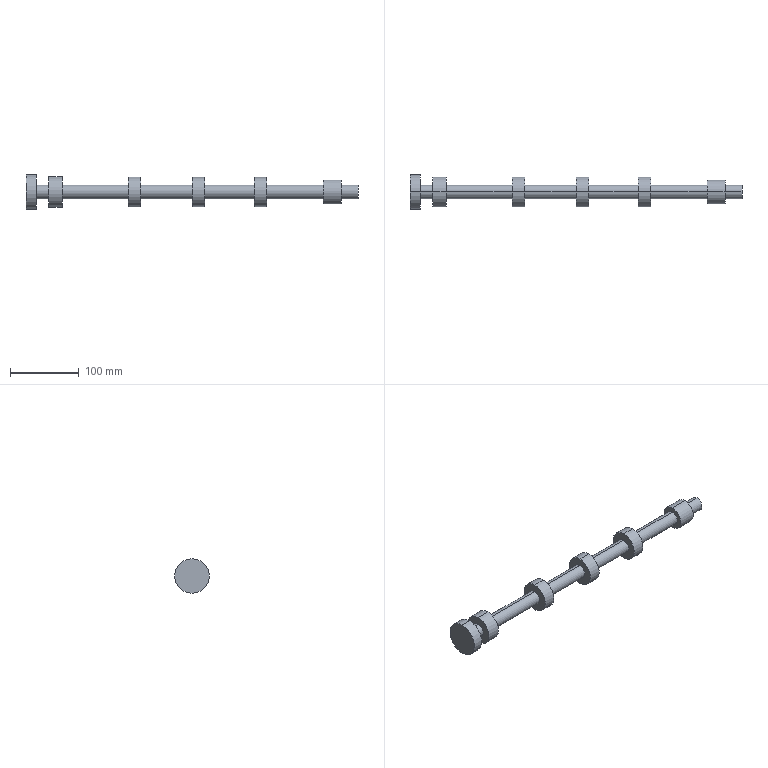Part | SolidWorks | features Revolution 1 | 1 solid | 37 faces | box 482.1 x 50 x 50 mm | volume 277870 mm3 | cylinder 24 | plane 13 | commonest cylinder face diameters 20 x12 34.5 x2 42.8 x2 43.1 x2 43.4 x2 43.7 x2
STEP:
#1=CARTESIAN_POINT('',(-2484.57,0.,10.));
#2=VERTEX_POINT('',#1);
#3=CARTESIAN_POINT('',(-2484.57,0.,-10.));
#4=VERTEX_POINT('',#3);
#5=CARTESIAN_POINT('',(-2484.57,0.,0.));
#6=DIRECTION('',(-1.,0.,0.));
#7=DIRECTION('',(0.,0.,1.));
#8=AXIS2_PLACEMENT_3D('',#5,#6,#7);
#9=CIRCLE('',#8,10.);
#10=EDGE_CURVE('',#2,#4,#9,.T.);
#11=ORIENTED_EDGE('',*,*,#10,.T.);
#12=CARTESIAN_POINT('',(-2509.17,0.,-10.));
#13=VERTEX_POINT('',#12);
#14=CARTESIAN_POINT('',(-2966.67,0.,-10.));
#15=DIRECTION('',(-1.,0.,0.));
#16=VECTOR('',#15,1000.);
#17=LINE('',#14,#16);
#18=EDGE_CURVE('',#4,#13,#17,.T.);
#19=ORIENTED_EDGE('',*,*,#18,.T.);
#20=CARTESIAN_POINT('',(-2509.17,0.,10.));
#21=VERTEX_POINT('',#20);
#22=CARTESIAN_POINT('',(-2509.17,0.,0.));
#23=DIRECTION('',(-1.,0.,0.));
#24=DIRECTION('',(0.,0.,1.));
#25=AXIS2_PLACEMENT_3D('',#22,#23,#24);
#26=CIRCLE('',#25,10.);
#27=EDGE_CURVE('',#21,#13,#26,.T.);
#28=ORIENTED_EDGE('',*,*,#27,.F.);
#29=CARTESIAN_POINT('',(-2966.67,0.,10.));
#30=DIRECTION('',(-1.,0.,0.));
#31=VECTOR('',#30,1000.);
#32=LINE('',#29,#31);
#33=EDGE_CURVE('',#2,#21,#32,.T.);
#34=ORIENTED_EDGE('',*,*,#33,.F.);
#35=EDGE_LOOP('',(#11,#19,#28,#34));
#36=FACE_OUTER_BOUND('',#35,.T.);
#37=CARTESIAN_POINT('',(-2966.67,0.,0.));
#38=DIRECTION('',(-1.,0.,0.));
#39=DIRECTION('',(0.,0.,1.));
#40=AXIS2_PLACEMENT_3D('',#37,#38,#39);
#41=CYLINDRICAL_SURFACE('',#40,10.);
#42=ADVANCED_FACE('',(#36),#41,.T.);
#43=CARTESIAN_POINT('',(-2509.17,0.,17.25));
#44=VERTEX_POINT('',#43);
#45=CARTESIAN_POINT('',(-2509.17,0.,-17.25));
#46=VERTEX_POINT('',#45);
#47=CARTESIAN_POINT('',(-2509.17,0.,0.));
#48=DIRECTION('',(-1.,0.,0.));
#49=DIRECTION('',(0.,0.,1.));
#50=AXIS2_PLACEMENT_3D('',#47,#48,#49);
#51=CIRCLE('',#50,17.25);
#52=EDGE_CURVE('',#44,#46,#51,.T.);
#53=ORIENTED_EDGE('',*,*,#52,.T.);
#54=CARTESIAN_POINT('',(-2535.17,0.,-17.25));
#55=VERTEX_POINT('',#54);
#56=CARTESIAN_POINT('',(-2966.67,0.,-17.25));
#57=DIRECTION('',(-1.,0.,0.));
#58=VECTOR('',#57,1000.);
#59=LINE('',#56,#58);
#60=EDGE_CURVE('',#46,#55,#59,.T.);
#61=ORIENTED_EDGE('',*,*,#60,.T.);
#62=CARTESIAN_POINT('',(-2535.17,0.,17.25));
#63=VERTEX_POINT('',#62);
#64=CARTESIAN_POINT('',(-2535.17,0.,0.));
#65=DIRECTION('',(-1.,0.,0.));
#66=DIRECTION('',(0.,0.,1.));
#67=AXIS2_PLACEMENT_3D('',#64,#65,#66);
#68=CIRCLE('',#67,17.25);
#69=EDGE_CURVE('',#63,#55,#68,.T.);
#70=ORIENTED_EDGE('',*,*,#69,.F.);
#71=CARTESIAN_POINT('',(-2966.67,0.,17.25));
#72=DIRECTION('',(-1.,0.,0.));
#73=VECTOR('',#72,1000.);
#74=LINE('',#71,#73);
#75=EDGE_CURVE('',#44,#63,#74,.T.);
#76=ORIENTED_EDGE('',*,*,#75,.F.);
#77=EDGE_LOOP('',(#53,#61,#70,#76));
#78=FACE_OUTER_BOUND('',#77,.T.);
#79=CARTESIAN_POINT('',(-2966.67,0.,0.));
#80=DIRECTION('',(-1.,0.,0.));
#81=DIRECTION('',(0.,0.,1.));
#82=AXIS2_PLACEMENT_3D('',#79,#80,#81);
#83=CYLINDRICAL_SURFACE('',#82,17.25);
#84=ADVANCED_FACE('',(#78),#83,.T.);
#85=CARTESIAN_POINT('',(-2535.17,0.,10.));
#86=VERTEX_POINT('',#85);
#87=CARTESIAN_POINT('',(-2535.17,0.,-10.));
#88=VERTEX_POINT('',#87);
#89=CARTESIAN_POINT('',(-2535.17,0.,0.));
#90=DIRECTION('',(-1.,0.,0.));
#91=DIRECTION('',(0.,0.,1.));
#92=AXIS2_PLACEMENT_3D('',#89,#90,#91);
#93=CIRCLE('',#92,10.);
#94=EDGE_CURVE('',#86,#88,#93,.T.);
#95=ORIENTED_EDGE('',*,*,#94,.T.);
#96=CARTESIAN_POINT('',(-2617.17,0.,-10.));
#97=VERTEX_POINT('',#96);
#98=CARTESIAN_POINT('',(-2966.67,0.,-10.));
#99=DIRECTION('',(-1.,0.,0.));
#100=VECTOR('',#99,1000.);
#101=LINE('',#98,#100);
#102=EDGE_CURVE('',#88,#97,#101,.T.);
#103=ORIENTED_EDGE('',*,*,#102,.T.);
#104=CARTESIAN_POINT('',(-2617.17,0.,10.));
#105=VERTEX_POINT('',#104);
#106=CARTESIAN_POINT('',(-2617.17,0.,0.));
#107=DIRECTION('',(-1.,0.,0.));
#108=DIRECTION('',(0.,0.,1.));
#109=AXIS2_PLACEMENT_3D('',#106,#107,#108);
#110=CIRCLE('',#109,10.);
#111=EDGE_CURVE('',#105,#97,#110,.T.);
#112=ORIENTED_EDGE('',*,*,#111,.F.);
#113=CARTESIAN_POINT('',(-2966.67,0.,10.));
#114=DIRECTION('',(-1.,0.,0.));
#115=VECTOR('',#114,1000.);
#116=LINE('',#113,#115);
#117=EDGE_CURVE('',#86,#105,#116,.T.);
#118=ORIENTED_EDGE('',*,*,#117,.F.);
#119=EDGE_LOOP('',(#95,#103,#112,#118));
#120=FACE_OUTER_BOUND('',#119,.T.);
#121=CARTESIAN_POINT('',(-2966.67,0.,0.));
#122=DIRECTION('',(-1.,0.,0.));
#123=DIRECTION('',(0.,0.,1.));
#124=AXIS2_PLACEMENT_3D('',#121,#122,#123);
#125=CYLINDRICAL_SURFACE('',#124,10.);
#126=ADVANCED_FACE('',(#120),#125,.T.);
#127=CARTESIAN_POINT('',(-2617.17,0.,21.4));
#128=VERTEX_POINT('',#127);
#129=CARTESIAN_POINT('',(-2617.17,0.,-21.4));
#130=VERTEX_POINT('',#129);
#131=CARTESIAN_POINT('',(-2617.17,0.,0.));
#132=DIRECTION('',(-1.,0.,0.));
#133=DIRECTION('',(0.,0.,1.));
#134=AXIS2_PLACEMENT_3D('',#131,#132,#133);
#135=CIRCLE('',#134,21.4);
#136=EDGE_CURVE('',#128,#130,#135,.T.);
#137=ORIENTED_EDGE('',*,*,#136,.T.);
#138=CARTESIAN_POINT('',(-2635.17,0.,-21.4));
#139=VERTEX_POINT('',#138);
#140=CARTESIAN_POINT('',(-2966.67,0.,-21.4));
#141=DIRECTION('',(-1.,0.,0.));
#142=VECTOR('',#141,1000.);
#143=LINE('',#140,#142);
#144=EDGE_CURVE('',#130,#139,#143,.T.);
#145=ORIENTED_EDGE('',*,*,#144,.T.);
#146=CARTESIAN_POINT('',(-2635.17,0.,21.4));
#147=VERTEX_POINT('',#146);
#148=CARTESIAN_POINT('',(-2635.17,0.,0.));
#149=DIRECTION('',(-1.,0.,0.));
#150=DIRECTION('',(0.,0.,1.));
#151=AXIS2_PLACEMENT_3D('',#148,#149,#150);
#152=CIRCLE('',#151,21.4);
#153=EDGE_CURVE('',#147,#139,#152,.T.);
#154=ORIENTED_EDGE('',*,*,#153,.F.);
#155=CARTESIAN_POINT('',(-2966.67,0.,21.4));
#156=DIRECTION('',(-1.,0.,0.));
#157=VECTOR('',#156,1000.);
#158=LINE('',#155,#157);
#159=EDGE_CURVE('',#128,#147,#158,.T.);
#160=ORIENTED_EDGE('',*,*,#159,.F.);
#161=EDGE_LOOP('',(#137,#145,#154,#160));
#162=FACE_OUTER_BOUND('',#161,.T.);
#163=CARTESIAN_POINT('',(-2966.67,0.,0.));
#164=DIRECTION('',(-1.,0.,0.));
#165=DIRECTION('',(0.,0.,1.));
#166=AXIS2_PLACEMENT_3D('',#163,#164,#165);
#167=CYLINDRICAL_SURFACE('',#166,21.4);
#168=ADVANCED_FACE('',(#162),#167,.T.);
#169=CARTESIAN_POINT('',(-2635.17,0.,10.));
#170=VERTEX_POINT('',#169);
#171=CARTESIAN_POINT('',(-2635.17,0.,-10.));
#172=VERTEX_POINT('',#171);
#173=CARTESIAN_POINT('',(-2635.17,0.,0.));
#174=DIRECTION('',(-1.,0.,0.));
#175=DIRECTION('',(0.,0.,1.));
#176=AXIS2_PLACEMENT_3D('',#173,#174,#175);
#177=CIRCLE('',#176,10.);
#178=EDGE_CURVE('',#170,#172,#177,.T.);
#179=ORIENTED_EDGE('',*,*,#178,.T.);
#180=CARTESIAN_POINT('',(-2707.17,0.,-10.));
#181=VERTEX_POINT('',#180);
#182=CARTESIAN_POINT('',(-2966.67,0.,-10.));
#183=DIRECTION('',(-1.,0.,0.));
#184=VECTOR('',#183,1000.);
#185=LINE('',#182,#184);
#186=EDGE_CURVE('',#172,#181,#185,.T.);
#187=ORIENTED_EDGE('',*,*,#186,.T.);
#188=CARTESIAN_POINT('',(-2707.17,0.,10.));
#189=VERTEX_POINT('',#188);
#190=CARTESIAN_POINT('',(-2707.17,0.,0.));
#191=DIRECTION('',(-1.,0.,0.));
#192=DIRECTION('',(0.,0.,1.));
#193=AXIS2_PLACEMENT_3D('',#190,#191,#192);
#194=CIRCLE('',#193,10.);
#195=EDGE_CURVE('',#189,#181,#194,.T.);
#196=ORIENTED_EDGE('',*,*,#195,.F.);
#197=CARTESIAN_POINT('',(-2966.67,0.,10.));
#198=DIRECTION('',(-1.,0.,0.));
#199=VECTOR('',#198,1000.);
#200=LINE('',#197,#199);
#201=EDGE_CURVE('',#170,#189,#200,.T.);
#202=ORIENTED_EDGE('',*,*,#201,.F.);
#203=EDGE_LOOP('',(#179,#187,#196,#202));
#204=FACE_OUTER_BOUND('',#203,.T.);
#205=CARTESIAN_POINT('',(-2966.67,0.,0.));
#206=DIRECTION('',(-1.,0.,0.));
#207=DIRECTION('',(0.,0.,1.));
#208=AXIS2_PLACEMENT_3D('',#205,#206,#207);
#209=CYLINDRICAL_SURFACE('',#208,10.);
#210=ADVANCED_FACE('',(#204),#209,.T.);
#211=CARTESIAN_POINT('',(-2707.17,0.,21.55));
#212=VERTEX_POINT('',#211);
#213=CARTESIAN_POINT('',(-2707.17,0.,-21.55));
#214=VERTEX_POINT('',#213);
#215=CARTESIAN_POINT('',(-2707.17,0.,0.));
#216=DIRECTION('',(-1.,0.,0.));
#217=DIRECTION('',(0.,0.,1.));
#218=AXIS2_PLACEMENT_3D('',#215,#216,#217);
#219=CIRCLE('',#218,21.55);
#220=EDGE_CURVE('',#212,#214,#219,.T.);
#221=ORIENTED_EDGE('',*,*,#220,.T.);
#222=CARTESIAN_POINT('',(-2725.17,0.,-21.55));
#223=VERTEX_POINT('',#222);
#224=CARTESIAN_POINT('',(-2966.67,0.,-21.55));
#225=DIRECTION('',(-1.,0.,0.));
#226=VECTOR('',#225,1000.);
#227=LINE('',#224,#226);
#228=EDGE_CURVE('',#214,#223,#227,.T.);
#229=ORIENTED_EDGE('',*,*,#228,.T.);
#230=CARTESIAN_POINT('',(-2725.17,0.,21.55));
#231=VERTEX_POINT('',#230);
#232=CARTESIAN_POINT('',(-2725.17,0.,0.));
#233=DIRECTION('',(-1.,0.,0.));
#234=DIRECTION('',(0.,0.,1.));
#235=AXIS2_PLACEMENT_3D('',#232,#233,#234);
#236=CIRCLE('',#235,21.55);
#237=EDGE_CURVE('',#231,#223,#236,.T.);
#238=ORIENTED_EDGE('',*,*,#237,.F.);
#239=CARTESIAN_POINT('',(-2966.67,0.,21.55));
#240=DIRECTION('',(-1.,0.,0.));
#241=VECTOR('',#240,1000.);
#242=LINE('',#239,#241);
#243=EDGE_CURVE('',#212,#231,#242,.T.);
#244=ORIENTED_EDGE('',*,*,#243,.F.);
#245=EDGE_LOOP('',(#221,#229,#238,#244));
#246=FACE_OUTER_BOUND('',#245,.T.);
#247=CARTESIAN_POINT('',(-2966.67,0.,0.));
#248=DIRECTION('',(-1.,0.,0.));
#249=DIRECTION('',(0.,0.,1.));
#250=AXIS2_PLACEMENT_3D('',#247,#248,#249);
#251=CYLINDRICAL_SURFACE('',#250,21.55);
#252=ADVANCED_FACE('',(#246),#251,.T.);
#253=CARTESIAN_POINT('',(-2725.17,0.,10.));
#254=VERTEX_POINT('',#253);
#255=CARTESIAN_POINT('',(-2725.17,0.,-10.));
#256=VERTEX_POINT('',#255);
#257=CARTESIAN_POINT('',(-2725.17,0.,0.));
#258=DIRECTION('',(-1.,0.,0.));
#259=DIRECTION('',(0.,0.,1.));
#260=AXIS2_PLACEMENT_3D('',#257,#258,#259);
#261=CIRCLE('',#260,10.);
#262=EDGE_CURVE('',#254,#256,#261,.T.);
#263=ORIENTED_EDGE('',*,*,#262,.T.);
#264=CARTESIAN_POINT('',(-2800.17,0.,-10.));
#265=VERTEX_POINT('',#264);
#266=CARTESIAN_POINT('',(-2966.67,0.,-10.));
#267=DIRECTION('',(-1.,0.,0.));
#268=VECTOR('',#267,1000.);
#269=LINE('',#266,#268);
#270=EDGE_CURVE('',#256,#265,#269,.T.);
#271=ORIENTED_EDGE('',*,*,#270,.T.);
#272=CARTESIAN_POINT('',(-2800.17,0.,10.));
#273=VERTEX_POINT('',#272);
#274=CARTESIAN_POINT('',(-2800.17,0.,0.));
#275=DIRECTION('',(-1.,0.,0.));
#276=DIRECTION('',(0.,0.,1.));
#277=AXIS2_PLACEMENT_3D('',#274,#275,#276);
#278=CIRCLE('',#277,10.);
#279=EDGE_CURVE('',#273,#265,#278,.T.);
#280=ORIENTED_EDGE('',*,*,#279,.F.);
#281=CARTESIAN_POINT('',(-2966.67,0.,10.));
#282=DIRECTION('',(-1.,0.,0.));
#283=VECTOR('',#282,1000.);
#284=LINE('',#281,#283);
#285=EDGE_CURVE('',#254,#273,#284,.T.);
#286=ORIENTED_EDGE('',*,*,#285,.F.);
#287=EDGE_LOOP('',(#263,#271,#280,#286));
#288=FACE_OUTER_BOUND('',#287,.T.);
#289=CARTESIAN_POINT('',(-2966.67,0.,0.));
#290=DIRECTION('',(-1.,0.,0.));
#291=DIRECTION('',(0.,0.,1.));
#292=AXIS2_PLACEMENT_3D('',#289,#290,#291);
#293=CYLINDRICAL_SURFACE('',#292,10.);
#294=ADVANCED_FACE('',(#288),#293,.T.);
#295=CARTESIAN_POINT('',(-2800.17,0.,21.7));
#296=VERTEX_POINT('',#295);
#297=CARTESIAN_POINT('',(-2800.17,0.,-21.7));
#298=VERTEX_POINT('',#297);
#299=CARTESIAN_POINT('',(-2800.17,0.,0.));
#300=DIRECTION('',(-1.,0.,0.));
#301=DIRECTION('',(0.,0.,1.));
#302=AXIS2_PLACEMENT_3D('',#299,#300,#301);
#303=CIRCLE('',#302,21.7);
#304=EDGE_CURVE('',#296,#298,#303,.T.);
#305=ORIENTED_EDGE('',*,*,#304,.T.);
#306=CARTESIAN_POINT('',(-2818.17,0.,-21.7));
#307=VERTEX_POINT('',#306);
#308=CARTESIAN_POINT('',(-2966.67,0.,-21.7));
#309=DIRECTION('',(-1.,0.,0.));
#310=VECTOR('',#309,1000.);
#311=LINE('',#308,#310);
#312=EDGE_CURVE('',#298,#307,#311,.T.);
#313=ORIENTED_EDGE('',*,*,#312,.T.);
#314=CARTESIAN_POINT('',(-2818.17,0.,21.7));
#315=VERTEX_POINT('',#314);
#316=CARTESIAN_POINT('',(-2818.17,0.,0.));
#317=DIRECTION('',(-1.,0.,0.));
#318=DIRECTION('',(0.,0.,1.));
#319=AXIS2_PLACEMENT_3D('',#316,#317,#318);
#320=CIRCLE('',#319,21.7);
#321=EDGE_CURVE('',#315,#307,#320,.T.);
#322=ORIENTED_EDGE('',*,*,#321,.F.);
#323=CARTESIAN_POINT('',(-2966.67,0.,21.7));
#324=DIRECTION('',(-1.,0.,0.));
#325=VECTOR('',#324,1000.);
#326=LINE('',#323,#325);
#327=EDGE_CURVE('',#296,#315,#326,.T.);
#328=ORIENTED_EDGE('',*,*,#327,.F.);
#329=EDGE_LOOP('',(#305,#313,#322,#328));
#330=FACE_OUTER_BOUND('',#329,.T.);
#331=CARTESIAN_POINT('',(-2966.67,0.,0.));
#332=DIRECTION('',(-1.,0.,0.));
#333=DIRECTION('',(0.,0.,1.));
#334=AXIS2_PLACEMENT_3D('',#331,#332,#333);
#335=CYLINDRICAL_SURFACE('',#334,21.7);
#336=ADVANCED_FACE('',(#330),#335,.T.);
#337=CARTESIAN_POINT('',(-2818.17,0.,10.));
#338=VERTEX_POINT('',#337);
#339=CARTESIAN_POINT('',(-2818.17,0.,-10.));
#340=VERTEX_POINT('',#339);
#341=CARTESIAN_POINT('',(-2818.17,0.,0.));
#342=DIRECTION('',(-1.,0.,0.));
#343=DIRECTION('',(0.,0.,1.));
#344=AXIS2_PLACEMENT_3D('',#341,#342,#343);
#345=CIRCLE('',#344,10.);
#346=EDGE_CURVE('',#338,#340,#345,.T.);
#347=ORIENTED_EDGE('',*,*,#346,.T.);
#348=CARTESIAN_POINT('',(-2913.92,0.,-10.));
#349=VERTEX_POINT('',#348);
#350=CARTESIAN_POINT('',(-2966.67,0.,-10.));
#351=DIRECTION('',(-1.,0.,0.));
#352=VECTOR('',#351,1000.);
#353=LINE('',#350,#352);
#354=EDGE_CURVE('',#340,#349,#353,.T.);
#355=ORIENTED_EDGE('',*,*,#354,.T.);
#356=CARTESIAN_POINT('',(-2913.92,0.,10.));
#357=VERTEX_POINT('',#356);
#358=CARTESIAN_POINT('',(-2913.92,0.,0.));
#359=DIRECTION('',(-1.,0.,0.));
#360=DIRECTION('',(0.,0.,1.));
#361=AXIS2_PLACEMENT_3D('',#358,#359,#360);
#362=CIRCLE('',#361,10.);
#363=EDGE_CURVE('',#357,#349,#362,.T.);
#364=ORIENTED_EDGE('',*,*,#363,.F.);
#365=CARTESIAN_POINT('',(-2966.67,0.,10.));
#366=DIRECTION('',(-1.,0.,0.));
#367=VECTOR('',#366,1000.);
#368=LINE('',#365,#367);
#369=EDGE_CURVE('',#338,#357,#368,.T.);
#370=ORIENTED_EDGE('',*,*,#369,.F.);
#371=EDGE_LOOP('',(#347,#355,#364,#370));
#372=FACE_OUTER_BOUND('',#371,.T.);
#373=CARTESIAN_POINT('',(-2966.67,0.,0.));
#374=DIRECTION('',(-1.,0.,0.));
#375=DIRECTION('',(0.,0.,1.));
#376=AXIS2_PLACEMENT_3D('',#373,#374,#375);
#377=CYLINDRICAL_SURFACE('',#376,10.);
#378=ADVANCED_FACE('',(#372),#377,.T.);
#379=CARTESIAN_POINT('',(-2913.92,0.,21.85));
#380=VERTEX_POINT('',#379);
#381=CARTESIAN_POINT('',(-2913.92,0.,-21.85));
#382=VERTEX_POINT('',#381);
#383=CARTESIAN_POINT('',(-2913.92,0.,0.));
#384=DIRECTION('',(-1.,0.,0.));
#385=DIRECTION('',(0.,0.,1.));
#386=AXIS2_PLACEMENT_3D('',#383,#384,#385);
#387=CIRCLE('',#386,21.85);
#388=EDGE_CURVE('',#380,#382,#387,.T.);
#389=ORIENTED_EDGE('',*,*,#388,.T.);
#390=CARTESIAN_POINT('',(-2933.92,0.,-21.85));
#391=VERTEX_POINT('',#390);
#392=CARTESIAN_POINT('',(-2966.67,0.,-21.85));
#393=DIRECTION('',(-1.,0.,0.));
#394=VECTOR('',#393,1000.);
#395=LINE('',#392,#394);
#396=EDGE_CURVE('',#382,#391,#395,.T.);
#397=ORIENTED_EDGE('',*,*,#396,.T.);
#398=CARTESIAN_POINT('',(-2933.92,0.,21.85));
#399=VERTEX_POINT('',#398);
#400=CARTESIAN_POINT('',(-2933.92,0.,0.));
#401=DIRECTION('',(-1.,0.,0.));
#402=DIRECTION('',(0.,0.,1.));
#403=AXIS2_PLACEMENT_3D('',#400,#401,#402);
#404=CIRCLE('',#403,21.85);
#405=EDGE_CURVE('',#399,#391,#404,.T.);
#406=ORIENTED_EDGE('',*,*,#405,.F.);
#407=CARTESIAN_POINT('',(-2966.67,0.,21.85));
#408=DIRECTION('',(-1.,0.,0.));
#409=VECTOR('',#408,1000.);
#410=LINE('',#407,#409);
#411=EDGE_CURVE('',#380,#399,#410,.T.);
#412=ORIENTED_EDGE('',*,*,#411,.F.);
#413=EDGE_LOOP('',(#389,#397,#406,#412));
#414=FACE_OUTER_BOUND('',#413,.T.);
#415=CARTESIAN_POINT('',(-2966.67,0.,0.));
#416=DIRECTION('',(-1.,0.,0.));
#417=DIRECTION('',(0.,0.,1.));
#418=AXIS2_PLACEMENT_3D('',#415,#416,#417);
#419=CYLINDRICAL_SURFACE('',#418,21.85);
#420=ADVANCED_FACE('',(#414),#419,.T.);
#421=CARTESIAN_POINT('',(-2933.92,0.,10.));
#422=VERTEX_POINT('',#421);
#423=CARTESIAN_POINT('',(-2933.92,0.,-10.));
#424=VERTEX_POINT('',#423);
#425=CARTESIAN_POINT('',(-2933.92,0.,0.));
#426=DIRECTION('',(-1.,0.,0.));
#427=DIRECTION('',(0.,0.,1.));
#428=AXIS2_PLACEMENT_3D('',#425,#426,#427);
#429=CIRCLE('',#428,10.);
#430=EDGE_CURVE('',#422,#424,#429,.T.);
#431=ORIENTED_EDGE('',*,*,#430,.T.);
#432=CARTESIAN_POINT('',(-2951.67,0.,-10.));
#433=VERTEX_POINT('',#432);
#434=CARTESIAN_POINT('',(-2966.67,0.,-10.));
#435=DIRECTION('',(-1.,0.,0.));
#436=VECTOR('',#435,1000.);
#437=LINE('',#434,#436);
#438=EDGE_CURVE('',#424,#433,#437,.T.);
#439=ORIENTED_EDGE('',*,*,#438,.T.);
#440=CARTESIAN_POINT('',(-2951.67,0.,10.));
#441=VERTEX_POINT('',#440);
#442=CARTESIAN_POINT('',(-2951.67,0.,0.));
#443=DIRECTION('',(-1.,0.,0.));
#444=DIRECTION('',(0.,0.,1.));
#445=AXIS2_PLACEMENT_3D('',#442,#443,#444);
#446=CIRCLE('',#445,10.);
#447=EDGE_CURVE('',#441,#433,#446,.T.);
#448=ORIENTED_EDGE('',*,*,#447,.F.);
#449=CARTESIAN_POINT('',(-2966.67,0.,10.));
#450=DIRECTION('',(-1.,0.,0.));
#451=VECTOR('',#450,1000.);
#452=LINE('',#449,#451);
#453=EDGE_CURVE('',#422,#441,#452,.T.);
#454=ORIENTED_EDGE('',*,*,#453,.F.);
#455=EDGE_LOOP('',(#431,#439,#448,#454));
#456=FACE_OUTER_BOUND('',#455,.T.);
#457=CARTESIAN_POINT('',(-2966.67,0.,0.));
#458=DIRECTION('',(-1.,0.,0.));
#459=DIRECTION('',(0.,0.,1.));
#460=AXIS2_PLACEMENT_3D('',#457,#458,#459);
#461=CYLINDRICAL_SURFACE('',#460,10.);
#462=ADVANCED_FACE('',(#456),#461,.T.);
#463=CARTESIAN_POINT('',(-2951.67,0.,25.));
#464=VERTEX_POINT('',#463);
#465=CARTESIAN_POINT('',(-2951.67,0.,-25.));
#466=VERTEX_POINT('',#465);
#467=CARTESIAN_POINT('',(-2951.67,0.,0.));
#468=DIRECTION('',(-1.,0.,0.));
#469=DIRECTION('',(0.,0.,1.));
#470=AXIS2_PLACEMENT_3D('',#467,#468,#469);
#471=CIRCLE('',#470,25.);
#472=EDGE_CURVE('',#464,#466,#471,.T.);
#473=ORIENTED_EDGE('',*,*,#472,.T.);
#474=CARTESIAN_POINT('',(-2966.67,0.,-25.));
#475=VERTEX_POINT('',#474);
#476=CARTESIAN_POINT('',(-2966.67,0.,-25.));
#477=DIRECTION('',(-1.,0.,0.));
#478=VECTOR('',#477,1000.);
#479=LINE('',#476,#478);
#480=EDGE_CURVE('',#466,#475,#479,.T.);
#481=ORIENTED_EDGE('',*,*,#480,.T.);
#482=CARTESIAN_POINT('',(-2966.67,0.,25.));
#483=VERTEX_POINT('',#482);
#484=CARTESIAN_POINT('',(-2966.67,0.,0.));
#485=DIRECTION('',(-1.,0.,0.));
#486=DIRECTION('',(0.,0.,1.));
#487=AXIS2_PLACEMENT_3D('',#484,#485,#486);
#488=CIRCLE('',#487,25.);
#489=EDGE_CURVE('',#483,#475,#488,.T.);
#490=ORIENTED_EDGE('',*,*,#489,.F.);
#491=CARTESIAN_POINT('',(-2966.67,0.,25.));
#492=DIRECTION('',(-1.,0.,0.));
#493=VECTOR('',#492,1000.);
#494=LINE('',#491,#493);
#495=EDGE_CURVE('',#464,#483,#494,.T.);
#496=ORIENTED_EDGE('',*,*,#495,.F.);
#497=EDGE_LOOP('',(#473,#481,#490,#496));
#498=FACE_OUTER_BOUND('',#497,.T.);
#499=CARTESIAN_POINT('',(-2966.67,0.,0.));
#500=DIRECTION('',(-1.,0.,0.));
#501=DIRECTION('',(0.,0.,1.));
#502=AXIS2_PLACEMENT_3D('',#499,#500,#501);
#503=CYLINDRICAL_SURFACE('',#502,25.);
#504=ADVANCED_FACE('',(#498),#503,.T.);
#505=ORIENTED_EDGE('',*,*,#489,.T.);
#506=CARTESIAN_POINT('',(-2966.67,0.,0.));
#507=DIRECTION('',(-1.,0.,0.));
#508=DIRECTION('',(0.,0.,1.));
#509=AXIS2_PLACEMENT_3D('',#506,#507,#508);
#510=CIRCLE('',#509,25.);
#511=EDGE_CURVE('',#475,#483,#510,.T.);
#512=ORIENTED_EDGE('',*,*,#511,.T.);
#513=EDGE_LOOP('',(#505,#512));
#514=FACE_OUTER_BOUND('',#513,.T.);
#515=CARTESIAN_POINT('',(-2966.67,0.,0.));
#516=DIRECTION('',(1.,0.,0.));
#517=DIRECTION('',(0.,0.,-1.));
#518=AXIS2_PLACEMENT_3D('',#515,#516,#517);
#519=PLANE('',#518);
#520=ADVANCED_FACE('',(#514),#519,.F.);
#521=ORIENTED_EDGE('',*,*,#480,.F.);
#522=CARTESIAN_POINT('',(-2951.67,0.,0.));
#523=DIRECTION('',(-1.,0.,0.));
#524=DIRECTION('',(0.,0.,1.));
#525=AXIS2_PLACEMENT_3D('',#522,#523,#524);
#526=CIRCLE('',#525,25.);
#527=EDGE_CURVE('',#466,#464,#526,.T.);
#528=ORIENTED_EDGE('',*,*,#527,.T.);
#529=ORIENTED_EDGE('',*,*,#495,.T.);
#530=ORIENTED_EDGE('',*,*,#511,.F.);
#531=EDGE_LOOP('',(#521,#528,#529,#530));
#532=FACE_OUTER_BOUND('',#531,.T.);
#533=CARTESIAN_POINT('',(-2966.67,0.,0.));
#534=DIRECTION('',(-1.,0.,0.));
#535=DIRECTION('',(0.,0.,1.));
#536=AXIS2_PLACEMENT_3D('',#533,#534,#535);
#537=CYLINDRICAL_SURFACE('',#536,25.);
#538=ADVANCED_FACE('',(#532),#537,.T.);
#539=ORIENTED_EDGE('',*,*,#472,.F.);
#540=ORIENTED_EDGE('',*,*,#527,.F.);
#541=EDGE_LOOP('',(#539,#540));
#542=FACE_OUTER_BOUND('',#541,.T.);
#543=ORIENTED_EDGE('',*,*,#447,.T.);
#544=CARTESIAN_POINT('',(-2951.67,0.,0.));
#545=DIRECTION('',(-1.,0.,0.));
#546=DIRECTION('',(0.,0.,1.));
#547=AXIS2_PLACEMENT_3D('',#544,#545,#546);
#548=CIRCLE('',#547,10.);
#549=EDGE_CURVE('',#433,#441,#548,.T.);
#550=ORIENTED_EDGE('',*,*,#549,.T.);
#551=EDGE_LOOP('',(#543,#550));
#552=FACE_BOUND('',#551,.T.);
#553=CARTESIAN_POINT('',(-2951.67,25.,0.));
#554=DIRECTION('',(-1.,0.,0.));
#555=DIRECTION('',(0.,0.,1.));
#556=AXIS2_PLACEMENT_3D('',#553,#554,#555);
#557=PLANE('',#556);
#558=ADVANCED_FACE('',(#542,#552),#557,.F.);
#559=ORIENTED_EDGE('',*,*,#438,.F.);
#560=CARTESIAN_POINT('',(-2933.92,0.,0.));
#561=DIRECTION('',(-1.,0.,0.));
#562=DIRECTION('',(0.,0.,1.));
#563=AXIS2_PLACEMENT_3D('',#560,#561,#562);
#564=CIRCLE('',#563,10.);
#565=EDGE_CURVE('',#424,#422,#564,.T.);
#566=ORIENTED_EDGE('',*,*,#565,.T.);
#567=ORIENTED_EDGE('',*,*,#453,.T.);
#568=ORIENTED_EDGE('',*,*,#549,.F.);
#569=EDGE_LOOP('',(#559,#566,#567,#568));
#570=FACE_OUTER_BOUND('',#569,.T.);
#571=CARTESIAN_POINT('',(-2966.67,0.,0.));
#572=DIRECTION('',(-1.,0.,0.));
#573=DIRECTION('',(0.,0.,1.));
#574=AXIS2_PLACEMENT_3D('',#571,#572,#573);
#575=CYLINDRICAL_SURFACE('',#574,10.);
#576=ADVANCED_FACE('',(#570),#575,.T.);
#577=ORIENTED_EDGE('',*,*,#430,.F.);
#578=ORIENTED_EDGE('',*,*,#565,.F.);
#579=EDGE_LOOP('',(#577,#578));
#580=FACE_BOUND('',#579,.T.);
#581=ORIENTED_EDGE('',*,*,#405,.T.);
#582=CARTESIAN_POINT('',(-2933.92,0.,0.));
#583=DIRECTION('',(-1.,0.,0.));
#584=DIRECTION('',(0.,0.,1.));
#585=AXIS2_PLACEMENT_3D('',#582,#583,#584);
#586=CIRCLE('',#585,21.85);
#587=EDGE_CURVE('',#391,#399,#586,.T.);
#588=ORIENTED_EDGE('',*,*,#587,.T.);
#589=EDGE_LOOP('',(#581,#588));
#590=FACE_OUTER_BOUND('',#589,.T.);
#591=CARTESIAN_POINT('',(-2933.92,10.,0.));
#592=DIRECTION('',(1.,0.,0.));
#593=DIRECTION('',(0.,0.,-1.));
#594=AXIS2_PLACEMENT_3D('',#591,#592,#593);
#595=PLANE('',#594);
#596=ADVANCED_FACE('',(#580,#590),#595,.F.);
#597=ORIENTED_EDGE('',*,*,#396,.F.);
#598=CARTESIAN_POINT('',(-2913.92,0.,0.));
#599=DIRECTION('',(-1.,0.,0.));
#600=DIRECTION('',(0.,0.,1.));
#601=AXIS2_PLACEMENT_3D('',#598,#599,#600);
#602=CIRCLE('',#601,21.85);
#603=EDGE_CURVE('',#382,#380,#602,.T.);
#604=ORIENTED_EDGE('',*,*,#603,.T.);
#605=ORIENTED_EDGE('',*,*,#411,.T.);
#606=ORIENTED_EDGE('',*,*,#587,.F.);
#607=EDGE_LOOP('',(#597,#604,#605,#606));
#608=FACE_OUTER_BOUND('',#607,.T.);
#609=CARTESIAN_POINT('',(-2966.67,0.,0.));
#610=DIRECTION('',(-1.,0.,0.));
#611=DIRECTION('',(0.,0.,1.));
#612=AXIS2_PLACEMENT_3D('',#609,#610,#611);
#613=CYLINDRICAL_SURFACE('',#612,21.85);
#614=ADVANCED_FACE('',(#608),#613,.T.);
#615=ORIENTED_EDGE('',*,*,#388,.F.);
#616=ORIENTED_EDGE('',*,*,#603,.F.);
#617=EDGE_LOOP('',(#615,#616));
#618=FACE_OUTER_BOUND('',#617,.T.);
#619=ORIENTED_EDGE('',*,*,#363,.T.);
#620=CARTESIAN_POINT('',(-2913.92,0.,0.));
#621=DIRECTION('',(-1.,0.,0.));
#622=DIRECTION('',(0.,0.,1.));
#623=AXIS2_PLACEMENT_3D('',#620,#621,#622);
#624=CIRCLE('',#623,10.);
#625=EDGE_CURVE('',#349,#357,#624,.T.);
#626=ORIENTED_EDGE('',*,*,#625,.T.);
#627=EDGE_LOOP('',(#619,#626));
#628=FACE_BOUND('',#627,.T.);
#629=CARTESIAN_POINT('',(-2913.92,21.85,0.));
#630=DIRECTION('',(-1.,0.,0.));
#631=DIRECTION('',(0.,0.,1.));
#632=AXIS2_PLACEMENT_3D('',#629,#630,#631);
#633=PLANE('',#632);
#634=ADVANCED_FACE('',(#618,#628),#633,.F.);
#635=ORIENTED_EDGE('',*,*,#354,.F.);
#636=CARTESIAN_POINT('',(-2818.17,0.,0.));
#637=DIRECTION('',(-1.,0.,0.));
#638=DIRECTION('',(0.,0.,1.));
#639=AXIS2_PLACEMENT_3D('',#636,#637,#638);
#640=CIRCLE('',#639,10.);
#641=EDGE_CURVE('',#340,#338,#640,.T.);
#642=ORIENTED_EDGE('',*,*,#641,.T.);
#643=ORIENTED_EDGE('',*,*,#369,.T.);
#644=ORIENTED_EDGE('',*,*,#625,.F.);
#645=EDGE_LOOP('',(#635,#642,#643,#644));
#646=FACE_OUTER_BOUND('',#645,.T.);
#647=CARTESIAN_POINT('',(-2966.67,0.,0.));
#648=DIRECTION('',(-1.,0.,0.));
#649=DIRECTION('',(0.,0.,1.));
#650=AXIS2_PLACEMENT_3D('',#647,#648,#649);
#651=CYLINDRICAL_SURFACE('',#650,10.);
#652=ADVANCED_FACE('',(#646),#651,.T.);
#653=ORIENTED_EDGE('',*,*,#346,.F.);
#654=ORIENTED_EDGE('',*,*,#641,.F.);
#655=EDGE_LOOP('',(#653,#654));
#656=FACE_BOUND('',#655,.T.);
#657=ORIENTED_EDGE('',*,*,#321,.T.);
#658=CARTESIAN_POINT('',(-2818.17,0.,0.));
#659=DIRECTION('',(-1.,0.,0.));
#660=DIRECTION('',(0.,0.,1.));
#661=AXIS2_PLACEMENT_3D('',#658,#659,#660);
#662=CIRCLE('',#661,21.7);
#663=EDGE_CURVE('',#307,#315,#662,.T.);
#664=ORIENTED_EDGE('',*,*,#663,.T.);
#665=EDGE_LOOP('',(#657,#664));
#666=FACE_OUTER_BOUND('',#665,.T.);
#667=CARTESIAN_POINT('',(-2818.17,10.,0.));
#668=DIRECTION('',(1.,0.,0.));
#669=DIRECTION('',(0.,0.,-1.));
#670=AXIS2_PLACEMENT_3D('',#667,#668,#669);
#671=PLANE('',#670);
#672=ADVANCED_FACE('',(#656,#666),#671,.F.);
#673=ORIENTED_EDGE('',*,*,#312,.F.);
#674=CARTESIAN_POINT('',(-2800.17,0.,0.));
#675=DIRECTION('',(-1.,0.,0.));
#676=DIRECTION('',(0.,0.,1.));
#677=AXIS2_PLACEMENT_3D('',#674,#675,#676);
#678=CIRCLE('',#677,21.7);
#679=EDGE_CURVE('',#298,#296,#678,.T.);
#680=ORIENTED_EDGE('',*,*,#679,.T.);
#681=ORIENTED_EDGE('',*,*,#327,.T.);
#682=ORIENTED_EDGE('',*,*,#663,.F.);
#683=EDGE_LOOP('',(#673,#680,#681,#682));
#684=FACE_OUTER_BOUND('',#683,.T.);
#685=CARTESIAN_POINT('',(-2966.67,0.,0.));
#686=DIRECTION('',(-1.,0.,0.));
#687=DIRECTION('',(0.,0.,1.));
#688=AXIS2_PLACEMENT_3D('',#685,#686,#687);
#689=CYLINDRICAL_SURFACE('',#688,21.7);
#690=ADVANCED_FACE('',(#684),#689,.T.);
#691=ORIENTED_EDGE('',*,*,#304,.F.);
#692=ORIENTED_EDGE('',*,*,#679,.F.);
#693=EDGE_LOOP('',(#691,#692));
#694=FACE_OUTER_BOUND('',#693,.T.);
#695=ORIENTED_EDGE('',*,*,#279,.T.);
#696=CARTESIAN_POINT('',(-2800.17,0.,0.));
#697=DIRECTION('',(-1.,0.,0.));
#698=DIRECTION('',(0.,0.,1.));
#699=AXIS2_PLACEMENT_3D('',#696,#697,#698);
#700=CIRCLE('',#699,10.);
#701=EDGE_CURVE('',#265,#273,#700,.T.);
#702=ORIENTED_EDGE('',*,*,#701,.T.);
#703=EDGE_LOOP('',(#695,#702));
#704=FACE_BOUND('',#703,.T.);
#705=CARTESIAN_POINT('',(-2800.17,21.7,0.));
#706=DIRECTION('',(-1.,0.,0.));
#707=DIRECTION('',(0.,0.,1.));
#708=AXIS2_PLACEMENT_3D('',#705,#706,#707);
#709=PLANE('',#708);
#710=ADVANCED_FACE('',(#694,#704),#709,.F.);
#711=ORIENTED_EDGE('',*,*,#270,.F.);
#712=CARTESIAN_POINT('',(-2725.17,0.,0.));
#713=DIRECTION('',(-1.,0.,0.));
#714=DIRECTION('',(0.,0.,1.));
#715=AXIS2_PLACEMENT_3D('',#712,#713,#714);
#716=CIRCLE('',#715,10.);
#717=EDGE_CURVE('',#256,#254,#716,.T.);
#718=ORIENTED_EDGE('',*,*,#717,.T.);
#719=ORIENTED_EDGE('',*,*,#285,.T.);
#720=ORIENTED_EDGE('',*,*,#701,.F.);
#721=EDGE_LOOP('',(#711,#718,#719,#720));
#722=FACE_OUTER_BOUND('',#721,.T.);
#723=CARTESIAN_POINT('',(-2966.67,0.,0.));
#724=DIRECTION('',(-1.,0.,0.));
#725=DIRECTION('',(0.,0.,1.));
#726=AXIS2_PLACEMENT_3D('',#723,#724,#725);
#727=CYLINDRICAL_SURFACE('',#726,10.);
#728=ADVANCED_FACE('',(#722),#727,.T.);
#729=ORIENTED_EDGE('',*,*,#262,.F.);
#730=ORIENTED_EDGE('',*,*,#717,.F.);
#731=EDGE_LOOP('',(#729,#730));
#732=FACE_BOUND('',#731,.T.);
#733=ORIENTED_EDGE('',*,*,#237,.T.);
#734=CARTESIAN_POINT('',(-2725.17,0.,0.));
#735=DIRECTION('',(-1.,0.,0.));
#736=DIRECTION('',(0.,0.,1.));
#737=AXIS2_PLACEMENT_3D('',#734,#735,#736);
#738=CIRCLE('',#737,21.55);
#739=EDGE_CURVE('',#223,#231,#738,.T.);
#740=ORIENTED_EDGE('',*,*,#739,.T.);
#741=EDGE_LOOP('',(#733,#740));
#742=FACE_OUTER_BOUND('',#741,.T.);
#743=CARTESIAN_POINT('',(-2725.17,10.,0.));
#744=DIRECTION('',(1.,0.,0.));
#745=DIRECTION('',(0.,0.,-1.));
#746=AXIS2_PLACEMENT_3D('',#743,#744,#745);
#747=PLANE('',#746);
#748=ADVANCED_FACE('',(#732,#742),#747,.F.);
#749=ORIENTED_EDGE('',*,*,#228,.F.);
#750=CARTESIAN_POINT('',(-2707.17,0.,0.));
#751=DIRECTION('',(-1.,0.,0.));
#752=DIRECTION('',(0.,0.,1.));
#753=AXIS2_PLACEMENT_3D('',#750,#751,#752);
#754=CIRCLE('',#753,21.55);
#755=EDGE_CURVE('',#214,#212,#754,.T.);
#756=ORIENTED_EDGE('',*,*,#755,.T.);
#757=ORIENTED_EDGE('',*,*,#243,.T.);
#758=ORIENTED_EDGE('',*,*,#739,.F.);
#759=EDGE_LOOP('',(#749,#756,#757,#758));
#760=FACE_OUTER_BOUND('',#759,.T.);
#761=CARTESIAN_POINT('',(-2966.67,0.,0.));
#762=DIRECTION('',(-1.,0.,0.));
#763=DIRECTION('',(0.,0.,1.));
#764=AXIS2_PLACEMENT_3D('',#761,#762,#763);
#765=CYLINDRICAL_SURFACE('',#764,21.55);
#766=ADVANCED_FACE('',(#760),#765,.T.);
#767=ORIENTED_EDGE('',*,*,#220,.F.);
#768=ORIENTED_EDGE('',*,*,#755,.F.);
#769=EDGE_LOOP('',(#767,#768));
#770=FACE_OUTER_BOUND('',#769,.T.);
#771=ORIENTED_EDGE('',*,*,#195,.T.);
#772=CARTESIAN_POINT('',(-2707.17,0.,0.));
#773=DIRECTION('',(-1.,0.,0.));
#774=DIRECTION('',(0.,0.,1.));
#775=AXIS2_PLACEMENT_3D('',#772,#773,#774);
#776=CIRCLE('',#775,10.);
#777=EDGE_CURVE('',#181,#189,#776,.T.);
#778=ORIENTED_EDGE('',*,*,#777,.T.);
#779=EDGE_LOOP('',(#771,#778));
#780=FACE_BOUND('',#779,.T.);
#781=CARTESIAN_POINT('',(-2707.17,21.55,0.));
#782=DIRECTION('',(-1.,0.,0.));
#783=DIRECTION('',(0.,0.,1.));
#784=AXIS2_PLACEMENT_3D('',#781,#782,#783);
#785=PLANE('',#784);
#786=ADVANCED_FACE('',(#770,#780),#785,.F.);
#787=ORIENTED_EDGE('',*,*,#186,.F.);
#788=CARTESIAN_POINT('',(-2635.17,0.,0.));
#789=DIRECTION('',(-1.,0.,0.));
#790=DIRECTION('',(0.,0.,1.));
#791=AXIS2_PLACEMENT_3D('',#788,#789,#790);
#792=CIRCLE('',#791,10.);
#793=EDGE_CURVE('',#172,#170,#792,.T.);
#794=ORIENTED_EDGE('',*,*,#793,.T.);
#795=ORIENTED_EDGE('',*,*,#201,.T.);
#796=ORIENTED_EDGE('',*,*,#777,.F.);
#797=EDGE_LOOP('',(#787,#794,#795,#796));
#798=FACE_OUTER_BOUND('',#797,.T.);
#799=CARTESIAN_POINT('',(-2966.67,0.,0.));
#800=DIRECTION('',(-1.,0.,0.));
#801=DIRECTION('',(0.,0.,1.));
#802=AXIS2_PLACEMENT_3D('',#799,#800,#801);
#803=CYLINDRICAL_SURFACE('',#802,10.);
#804=ADVANCED_FACE('',(#798),#803,.T.);
#805=ORIENTED_EDGE('',*,*,#178,.F.);
#806=ORIENTED_EDGE('',*,*,#793,.F.);
#807=EDGE_LOOP('',(#805,#806));
#808=FACE_BOUND('',#807,.T.);
#809=ORIENTED_EDGE('',*,*,#153,.T.);
#810=CARTESIAN_POINT('',(-2635.17,0.,0.));
#811=DIRECTION('',(-1.,0.,0.));
#812=DIRECTION('',(0.,0.,1.));
#813=AXIS2_PLACEMENT_3D('',#810,#811,#812);
#814=CIRCLE('',#813,21.4);
#815=EDGE_CURVE('',#139,#147,#814,.T.);
#816=ORIENTED_EDGE('',*,*,#815,.T.);
#817=EDGE_LOOP('',(#809,#816));
#818=FACE_OUTER_BOUND('',#817,.T.);
#819=CARTESIAN_POINT('',(-2635.17,10.,0.));
#820=DIRECTION('',(1.,0.,0.));
#821=DIRECTION('',(0.,0.,-1.));
#822=AXIS2_PLACEMENT_3D('',#819,#820,#821);
#823=PLANE('',#822);
#824=ADVANCED_FACE('',(#808,#818),#823,.F.);
#825=ORIENTED_EDGE('',*,*,#144,.F.);
#826=CARTESIAN_POINT('',(-2617.17,0.,0.));
#827=DIRECTION('',(-1.,0.,0.));
#828=DIRECTION('',(0.,0.,1.));
#829=AXIS2_PLACEMENT_3D('',#826,#827,#828);
#830=CIRCLE('',#829,21.4);
#831=EDGE_CURVE('',#130,#128,#830,.T.);
#832=ORIENTED_EDGE('',*,*,#831,.T.);
#833=ORIENTED_EDGE('',*,*,#159,.T.);
#834=ORIENTED_EDGE('',*,*,#815,.F.);
#835=EDGE_LOOP('',(#825,#832,#833,#834));
#836=FACE_OUTER_BOUND('',#835,.T.);
#837=CARTESIAN_POINT('',(-2966.67,0.,0.));
#838=DIRECTION('',(-1.,0.,0.));
#839=DIRECTION('',(0.,0.,1.));
#840=AXIS2_PLACEMENT_3D('',#837,#838,#839);
#841=CYLINDRICAL_SURFACE('',#840,21.4);
#842=ADVANCED_FACE('',(#836),#841,.T.);
#843=ORIENTED_EDGE('',*,*,#136,.F.);
#844=ORIENTED_EDGE('',*,*,#831,.F.);
#845=EDGE_LOOP('',(#843,#844));
#846=FACE_OUTER_BOUND('',#845,.T.);
#847=ORIENTED_EDGE('',*,*,#111,.T.);
#848=CARTESIAN_POINT('',(-2617.17,0.,0.));
#849=DIRECTION('',(-1.,0.,0.));
#850=DIRECTION('',(0.,0.,1.));
#851=AXIS2_PLACEMENT_3D('',#848,#849,#850);
#852=CIRCLE('',#851,10.);
#853=EDGE_CURVE('',#97,#105,#852,.T.);
#854=ORIENTED_EDGE('',*,*,#853,.T.);
#855=EDGE_LOOP('',(#847,#854));
#856=FACE_BOUND('',#855,.T.);
#857=CARTESIAN_POINT('',(-2617.17,21.4,0.));
#858=DIRECTION('',(-1.,0.,0.));
#859=DIRECTION('',(0.,0.,1.));
#860=AXIS2_PLACEMENT_3D('',#857,#858,#859);
#861=PLANE('',#860);
#862=ADVANCED_FACE('',(#846,#856),#861,.F.);
#863=ORIENTED_EDGE('',*,*,#102,.F.);
#864=CARTESIAN_POINT('',(-2535.17,0.,0.));
#865=DIRECTION('',(-1.,0.,0.));
#866=DIRECTION('',(0.,0.,1.));
#867=AXIS2_PLACEMENT_3D('',#864,#865,#866);
#868=CIRCLE('',#867,10.);
#869=EDGE_CURVE('',#88,#86,#868,.T.);
#870=ORIENTED_EDGE('',*,*,#869,.T.);
#871=ORIENTED_EDGE('',*,*,#117,.T.);
#872=ORIENTED_EDGE('',*,*,#853,.F.);
#873=EDGE_LOOP('',(#863,#870,#871,#872));
#874=FACE_OUTER_BOUND('',#873,.T.);
#875=CARTESIAN_POINT('',(-2966.67,0.,0.));
#876=DIRECTION('',(-1.,0.,0.));
#877=DIRECTION('',(0.,0.,1.));
#878=AXIS2_PLACEMENT_3D('',#875,#876,#877);
#879=CYLINDRICAL_SURFACE('',#878,10.);
#880=ADVANCED_FACE('',(#874),#879,.T.);
#881=ORIENTED_EDGE('',*,*,#94,.F.);
#882=ORIENTED_EDGE('',*,*,#869,.F.);
#883=EDGE_LOOP('',(#881,#882));
#884=FACE_BOUND('',#883,.T.);
#885=ORIENTED_EDGE('',*,*,#69,.T.);
#886=CARTESIAN_POINT('',(-2535.17,0.,0.));
#887=DIRECTION('',(-1.,0.,0.));
#888=DIRECTION('',(0.,0.,1.));
#889=AXIS2_PLACEMENT_3D('',#886,#887,#888);
#890=CIRCLE('',#889,17.25);
#891=EDGE_CURVE('',#55,#63,#890,.T.);
#892=ORIENTED_EDGE('',*,*,#891,.T.);
#893=EDGE_LOOP('',(#885,#892));
#894=FACE_OUTER_BOUND('',#893,.T.);
#895=CARTESIAN_POINT('',(-2535.17,10.,0.));
#896=DIRECTION('',(1.,0.,0.));
#897=DIRECTION('',(0.,0.,-1.));
#898=AXIS2_PLACEMENT_3D('',#895,#896,#897);
#899=PLANE('',#898);
#900=ADVANCED_FACE('',(#884,#894),#899,.F.);
#901=ORIENTED_EDGE('',*,*,#60,.F.);
#902=CARTESIAN_POINT('',(-2509.17,0.,0.));
#903=DIRECTION('',(-1.,0.,0.));
#904=DIRECTION('',(0.,0.,1.));
#905=AXIS2_PLACEMENT_3D('',#902,#903,#904);
#906=CIRCLE('',#905,17.25);
#907=EDGE_CURVE('',#46,#44,#906,.T.);
#908=ORIENTED_EDGE('',*,*,#907,.T.);
#909=ORIENTED_EDGE('',*,*,#75,.T.);
#910=ORIENTED_EDGE('',*,*,#891,.F.);
#911=EDGE_LOOP('',(#901,#908,#909,#910));
#912=FACE_OUTER_BOUND('',#911,.T.);
#913=CARTESIAN_POINT('',(-2966.67,0.,0.));
#914=DIRECTION('',(-1.,0.,0.));
#915=DIRECTION('',(0.,0.,1.));
#916=AXIS2_PLACEMENT_3D('',#913,#914,#915);
#917=CYLINDRICAL_SURFACE('',#916,17.25);
#918=ADVANCED_FACE('',(#912),#917,.T.);
#919=ORIENTED_EDGE('',*,*,#52,.F.);
#920=ORIENTED_EDGE('',*,*,#907,.F.);
#921=EDGE_LOOP('',(#919,#920));
#922=FACE_OUTER_BOUND('',#921,.T.);
#923=ORIENTED_EDGE('',*,*,#27,.T.);
#924=CARTESIAN_POINT('',(-2509.17,0.,0.));
#925=DIRECTION('',(-1.,0.,0.));
#926=DIRECTION('',(0.,0.,1.));
#927=AXIS2_PLACEMENT_3D('',#924,#925,#926);
#928=CIRCLE('',#927,10.);
#929=EDGE_CURVE('',#13,#21,#928,.T.);
#930=ORIENTED_EDGE('',*,*,#929,.T.);
#931=EDGE_LOOP('',(#923,#930));
#932=FACE_BOUND('',#931,.T.);
#933=CARTESIAN_POINT('',(-2509.17,17.25,0.));
#934=DIRECTION('',(-1.,0.,0.));
#935=DIRECTION('',(0.,0.,1.));
#936=AXIS2_PLACEMENT_3D('',#933,#934,#935);
#937=PLANE('',#936);
#938=ADVANCED_FACE('',(#922,#932),#937,.F.);
#939=ORIENTED_EDGE('',*,*,#18,.F.);
#940=CARTESIAN_POINT('',(-2484.57,0.,0.));
#941=DIRECTION('',(-1.,0.,0.));
#942=DIRECTION('',(0.,0.,1.));
#943=AXIS2_PLACEMENT_3D('',#940,#941,#942);
#944=CIRCLE('',#943,10.);
#945=EDGE_CURVE('',#4,#2,#944,.T.);
#946=ORIENTED_EDGE('',*,*,#945,.T.);
#947=ORIENTED_EDGE('',*,*,#33,.T.);
#948=ORIENTED_EDGE('',*,*,#929,.F.);
#949=EDGE_LOOP('',(#939,#946,#947,#948));
#950=FACE_OUTER_BOUND('',#949,.T.);
#951=CARTESIAN_POINT('',(-2966.67,0.,0.));
#952=DIRECTION('',(-1.,0.,0.));
#953=DIRECTION('',(0.,0.,1.));
#954=AXIS2_PLACEMENT_3D('',#951,#952,#953);
#955=CYLINDRICAL_SURFACE('',#954,10.);
#956=ADVANCED_FACE('',(#950),#955,.T.);
#957=ORIENTED_EDGE('',*,*,#10,.F.);
#958=ORIENTED_EDGE('',*,*,#945,.F.);
#959=EDGE_LOOP('',(#957,#958));
#960=FACE_OUTER_BOUND('',#959,.T.);
#961=CARTESIAN_POINT('',(-2484.57,10.,0.));
#962=DIRECTION('',(-1.,0.,0.));
#963=DIRECTION('',(0.,0.,1.));
#964=AXIS2_PLACEMENT_3D('',#961,#962,#963);
#965=PLANE('',#964);
#966=ADVANCED_FACE('',(#960),#965,.F.);
#967=CLOSED_SHELL('',(#42,#84,#126,#168,#210,#252,#294,#336,#378,#420,#462,#504,#520,#538,#558,#576,#596,#614,#634,#652,#672,#690,#710,#728,#748,#766,#786,#804,#824,#842,#862,#880,#900,#918,#938,#956,#966));
#968=MANIFOLD_SOLID_BREP('',#967);
#969=CARTESIAN_POINT('',(0.,0.,0.));
#970=DIRECTION('',(0.,0.,1.));
#971=DIRECTION('',(1.,0.,0.));
#972=AXIS2_PLACEMENT_3D('',#969,#970,#971);
#973=(LENGTH_UNIT()NAMED_UNIT(*)SI_UNIT(.MILLI.,.METRE.));
#974=UNCERTAINTY_MEASURE_WITH_UNIT(LENGTH_MEASURE(0.00001),#973,'','');
#975=(NAMED_UNIT(*)PLANE_ANGLE_UNIT()SI_UNIT($,.RADIAN.));
#976=(NAMED_UNIT(*)SI_UNIT($,.STERADIAN.)SOLID_ANGLE_UNIT());
#977=(GEOMETRIC_REPRESENTATION_CONTEXT(3)GLOBAL_UNCERTAINTY_ASSIGNED_CONTEXT((#974))GLOBAL_UNIT_ASSIGNED_CONTEXT((#973,#975,#976))REPRESENTATION_CONTEXT('',''));
#978=ADVANCED_BREP_SHAPE_REPRESENTATION('',(#968,#972),#977);